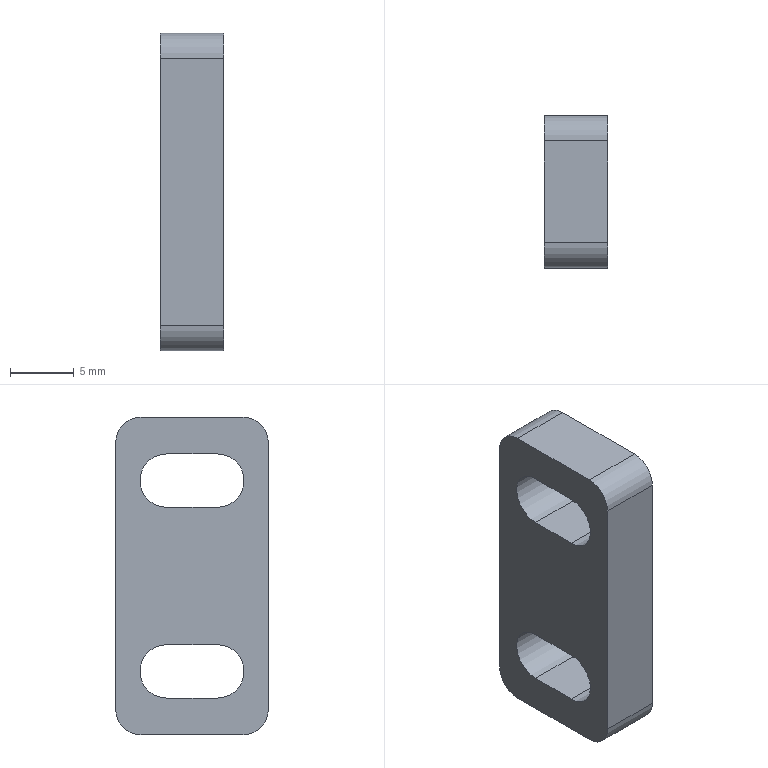Part | SolidWorks | features Fillet 4, ICE 4, Cut 1, Extrusion 1, HoleWzd 1 | 1 solid | 18 faces | box 5 x 12 x 25 mm | volume 1176 mm3 | plane 10 | cylinder 8 | commonest cylinder face diameters 4 x4 4.2 x4
STEP:
#1=CARTESIAN_POINT('',(0.,-4.,-12.5));
#2=VERTEX_POINT('',#1);
#3=CARTESIAN_POINT('',(0.,4.,-12.5));
#4=VERTEX_POINT('',#3);
#5=CARTESIAN_POINT('',(0.,6.,-12.5));
#6=DIRECTION('',(0.,1.,0.));
#7=VECTOR('',#6,1000.);
#8=LINE('',#5,#7);
#9=EDGE_CURVE('',#2,#4,#8,.T.);
#10=ORIENTED_EDGE('',*,*,#9,.T.);
#11=CARTESIAN_POINT('',(5.,4.,-12.5));
#12=VERTEX_POINT('',#11);
#13=CARTESIAN_POINT('',(5.,4.,-12.5));
#14=DIRECTION('',(1.,0.,0.));
#15=VECTOR('',#14,1000.);
#16=LINE('',#13,#15);
#17=EDGE_CURVE('',#4,#12,#16,.T.);
#18=ORIENTED_EDGE('',*,*,#17,.T.);
#19=CARTESIAN_POINT('',(5.,-4.,-12.5));
#20=VERTEX_POINT('',#19);
#21=CARTESIAN_POINT('',(5.,6.,-12.5));
#22=DIRECTION('',(0.,1.,0.));
#23=VECTOR('',#22,1000.);
#24=LINE('',#21,#23);
#25=EDGE_CURVE('',#20,#12,#24,.T.);
#26=ORIENTED_EDGE('',*,*,#25,.F.);
#27=CARTESIAN_POINT('',(5.,-4.,-12.5));
#28=DIRECTION('',(-1.,0.,0.));
#29=VECTOR('',#28,1000.);
#30=LINE('',#27,#29);
#31=EDGE_CURVE('',#20,#2,#30,.T.);
#32=ORIENTED_EDGE('',*,*,#31,.T.);
#33=EDGE_LOOP('',(#10,#18,#26,#32));
#34=FACE_OUTER_BOUND('',#33,.T.);
#35=CARTESIAN_POINT('',(5.,6.,-12.5));
#36=DIRECTION('',(0.,0.,1.));
#37=DIRECTION('',(0.,-1.,0.));
#38=AXIS2_PLACEMENT_3D('',#35,#36,#37);
#39=PLANE('',#38);
#40=ADVANCED_FACE('',(#34),#39,.F.);
#41=CARTESIAN_POINT('',(5.,4.,12.5));
#42=VERTEX_POINT('',#41);
#43=CARTESIAN_POINT('',(5.,-4.,12.5));
#44=VERTEX_POINT('',#43);
#45=CARTESIAN_POINT('',(5.,6.,12.5));
#46=DIRECTION('',(0.,-1.,0.));
#47=VECTOR('',#46,1000.);
#48=LINE('',#45,#47);
#49=EDGE_CURVE('',#42,#44,#48,.T.);
#50=ORIENTED_EDGE('',*,*,#49,.F.);
#51=CARTESIAN_POINT('',(0.,4.,12.5));
#52=VERTEX_POINT('',#51);
#53=CARTESIAN_POINT('',(5.,4.,12.5));
#54=DIRECTION('',(-1.,0.,0.));
#55=VECTOR('',#54,1000.);
#56=LINE('',#53,#55);
#57=EDGE_CURVE('',#42,#52,#56,.T.);
#58=ORIENTED_EDGE('',*,*,#57,.T.);
#59=CARTESIAN_POINT('',(0.,-4.,12.5));
#60=VERTEX_POINT('',#59);
#61=CARTESIAN_POINT('',(0.,6.,12.5));
#62=DIRECTION('',(0.,-1.,0.));
#63=VECTOR('',#62,1000.);
#64=LINE('',#61,#63);
#65=EDGE_CURVE('',#52,#60,#64,.T.);
#66=ORIENTED_EDGE('',*,*,#65,.T.);
#67=CARTESIAN_POINT('',(5.,-4.,12.5));
#68=DIRECTION('',(1.,0.,0.));
#69=VECTOR('',#68,1000.);
#70=LINE('',#67,#69);
#71=EDGE_CURVE('',#60,#44,#70,.T.);
#72=ORIENTED_EDGE('',*,*,#71,.T.);
#73=EDGE_LOOP('',(#50,#58,#66,#72));
#74=FACE_OUTER_BOUND('',#73,.T.);
#75=CARTESIAN_POINT('',(5.,6.,12.5));
#76=DIRECTION('',(0.,0.,-1.));
#77=DIRECTION('',(-1.,0.,0.));
#78=AXIS2_PLACEMENT_3D('',#75,#76,#77);
#79=PLANE('',#78);
#80=ADVANCED_FACE('',(#74),#79,.F.);
#81=CARTESIAN_POINT('',(0.,-6.,10.5));
#82=VERTEX_POINT('',#81);
#83=CARTESIAN_POINT('',(0.,-6.,-10.5));
#84=VERTEX_POINT('',#83);
#85=CARTESIAN_POINT('',(0.,-6.,12.5));
#86=DIRECTION('',(0.,0.,-1.));
#87=VECTOR('',#86,1000.);
#88=LINE('',#85,#87);
#89=EDGE_CURVE('',#82,#84,#88,.T.);
#90=ORIENTED_EDGE('',*,*,#89,.T.);
#91=CARTESIAN_POINT('',(5.,-6.,-10.5));
#92=VERTEX_POINT('',#91);
#93=CARTESIAN_POINT('',(5.,-6.,-10.5));
#94=DIRECTION('',(1.,0.,0.));
#95=VECTOR('',#94,1000.);
#96=LINE('',#93,#95);
#97=EDGE_CURVE('',#84,#92,#96,.T.);
#98=ORIENTED_EDGE('',*,*,#97,.T.);
#99=CARTESIAN_POINT('',(5.,-6.,10.5));
#100=VERTEX_POINT('',#99);
#101=CARTESIAN_POINT('',(5.,-6.,12.5));
#102=DIRECTION('',(0.,0.,-1.));
#103=VECTOR('',#102,1000.);
#104=LINE('',#101,#103);
#105=EDGE_CURVE('',#100,#92,#104,.T.);
#106=ORIENTED_EDGE('',*,*,#105,.F.);
#107=CARTESIAN_POINT('',(5.,-6.,10.5));
#108=DIRECTION('',(-1.,0.,0.));
#109=VECTOR('',#108,1000.);
#110=LINE('',#107,#109);
#111=EDGE_CURVE('',#100,#82,#110,.T.);
#112=ORIENTED_EDGE('',*,*,#111,.T.);
#113=EDGE_LOOP('',(#90,#98,#106,#112));
#114=FACE_OUTER_BOUND('',#113,.T.);
#115=CARTESIAN_POINT('',(5.,-6.,12.5));
#116=DIRECTION('',(0.,1.,0.));
#117=DIRECTION('',(0.,0.,1.));
#118=AXIS2_PLACEMENT_3D('',#115,#116,#117);
#119=PLANE('',#118);
#120=ADVANCED_FACE('',(#114),#119,.F.);
#121=CARTESIAN_POINT('',(5.,6.,10.5));
#122=VERTEX_POINT('',#121);
#123=CARTESIAN_POINT('',(5.,6.,-10.5));
#124=VERTEX_POINT('',#123);
#125=CARTESIAN_POINT('',(5.,6.,-15.392));
#126=DIRECTION('',(0.,0.,-1.));
#127=VECTOR('',#126,1000.);
#128=LINE('',#125,#127);
#129=EDGE_CURVE('',#122,#124,#128,.T.);
#130=ORIENTED_EDGE('',*,*,#129,.F.);
#131=CARTESIAN_POINT('',(5.,4.,10.5));
#132=DIRECTION('',(1.,0.,0.));
#133=DIRECTION('',(0.,0.,-1.));
#134=AXIS2_PLACEMENT_3D('',#131,#132,#133);
#135=CIRCLE('',#134,2.);
#136=EDGE_CURVE('',#122,#42,#135,.T.);
#137=ORIENTED_EDGE('',*,*,#136,.T.);
#138=ORIENTED_EDGE('',*,*,#49,.T.);
#139=CARTESIAN_POINT('',(5.,-4.,10.5));
#140=DIRECTION('',(1.,0.,0.));
#141=DIRECTION('',(0.,0.,-1.));
#142=AXIS2_PLACEMENT_3D('',#139,#140,#141);
#143=CIRCLE('',#142,2.);
#144=EDGE_CURVE('',#44,#100,#143,.T.);
#145=ORIENTED_EDGE('',*,*,#144,.T.);
#146=ORIENTED_EDGE('',*,*,#105,.T.);
#147=CARTESIAN_POINT('',(5.,-4.,-10.5));
#148=DIRECTION('',(1.,0.,0.));
#149=DIRECTION('',(0.,0.,-1.));
#150=AXIS2_PLACEMENT_3D('',#147,#148,#149);
#151=CIRCLE('',#150,2.);
#152=EDGE_CURVE('',#92,#20,#151,.T.);
#153=ORIENTED_EDGE('',*,*,#152,.T.);
#154=ORIENTED_EDGE('',*,*,#25,.T.);
#155=CARTESIAN_POINT('',(5.,4.,-10.5));
#156=DIRECTION('',(1.,0.,0.));
#157=DIRECTION('',(0.,0.,-1.));
#158=AXIS2_PLACEMENT_3D('',#155,#156,#157);
#159=CIRCLE('',#158,2.);
#160=EDGE_CURVE('',#12,#124,#159,.T.);
#161=ORIENTED_EDGE('',*,*,#160,.T.);
#162=EDGE_LOOP('',(#130,#137,#138,#145,#146,#153,#154,#161));
#163=FACE_OUTER_BOUND('',#162,.T.);
#164=CARTESIAN_POINT('',(5.,2.,5.4));
#165=VERTEX_POINT('',#164);
#166=CARTESIAN_POINT('',(5.,2.,9.6));
#167=VERTEX_POINT('',#166);
#168=CARTESIAN_POINT('',(5.,2.,7.5));
#169=DIRECTION('',(1.,0.,0.));
#170=DIRECTION('',(0.,0.,-1.));
#171=AXIS2_PLACEMENT_3D('',#168,#169,#170);
#172=CIRCLE('',#171,2.1);
#173=EDGE_CURVE('',#165,#167,#172,.T.);
#174=ORIENTED_EDGE('',*,*,#173,.F.);
#175=CARTESIAN_POINT('',(5.,-2.,5.4));
#176=VERTEX_POINT('',#175);
#177=CARTESIAN_POINT('',(5.,0.,5.4));
#178=DIRECTION('',(0.,1.,0.));
#179=VECTOR('',#178,1000.);
#180=LINE('',#177,#179);
#181=EDGE_CURVE('',#176,#165,#180,.T.);
#182=ORIENTED_EDGE('',*,*,#181,.F.);
#183=CARTESIAN_POINT('',(5.,-2.,9.6));
#184=VERTEX_POINT('',#183);
#185=CARTESIAN_POINT('',(5.,-2.,7.5));
#186=DIRECTION('',(1.,0.,0.));
#187=DIRECTION('',(0.,0.,-1.));
#188=AXIS2_PLACEMENT_3D('',#185,#186,#187);
#189=CIRCLE('',#188,2.1);
#190=EDGE_CURVE('',#184,#176,#189,.T.);
#191=ORIENTED_EDGE('',*,*,#190,.F.);
#192=CARTESIAN_POINT('',(5.,0.,9.6));
#193=DIRECTION('',(0.,-1.,0.));
#194=VECTOR('',#193,1000.);
#195=LINE('',#192,#194);
#196=EDGE_CURVE('',#167,#184,#195,.T.);
#197=ORIENTED_EDGE('',*,*,#196,.F.);
#198=EDGE_LOOP('',(#174,#182,#191,#197));
#199=FACE_BOUND('',#198,.T.);
#200=CARTESIAN_POINT('',(5.,2.,-9.6));
#201=VERTEX_POINT('',#200);
#202=CARTESIAN_POINT('',(5.,2.,-5.4));
#203=VERTEX_POINT('',#202);
#204=CARTESIAN_POINT('',(5.,2.,-7.5));
#205=DIRECTION('',(1.,0.,0.));
#206=DIRECTION('',(0.,0.,-1.));
#207=AXIS2_PLACEMENT_3D('',#204,#205,#206);
#208=CIRCLE('',#207,2.1);
#209=EDGE_CURVE('',#201,#203,#208,.T.);
#210=ORIENTED_EDGE('',*,*,#209,.F.);
#211=CARTESIAN_POINT('',(5.,-2.,-9.6));
#212=VERTEX_POINT('',#211);
#213=CARTESIAN_POINT('',(5.,0.,-9.6));
#214=DIRECTION('',(0.,1.,0.));
#215=VECTOR('',#214,1000.);
#216=LINE('',#213,#215);
#217=EDGE_CURVE('',#212,#201,#216,.T.);
#218=ORIENTED_EDGE('',*,*,#217,.F.);
#219=CARTESIAN_POINT('',(5.,-2.,-5.4));
#220=VERTEX_POINT('',#219);
#221=CARTESIAN_POINT('',(5.,-2.,-7.5));
#222=DIRECTION('',(1.,0.,0.));
#223=DIRECTION('',(0.,0.,-1.));
#224=AXIS2_PLACEMENT_3D('',#221,#222,#223);
#225=CIRCLE('',#224,2.1);
#226=EDGE_CURVE('',#220,#212,#225,.T.);
#227=ORIENTED_EDGE('',*,*,#226,.F.);
#228=CARTESIAN_POINT('',(5.,0.,-5.4));
#229=DIRECTION('',(0.,-1.,0.));
#230=VECTOR('',#229,1000.);
#231=LINE('',#228,#230);
#232=EDGE_CURVE('',#203,#220,#231,.T.);
#233=ORIENTED_EDGE('',*,*,#232,.F.);
#234=EDGE_LOOP('',(#210,#218,#227,#233));
#235=FACE_BOUND('',#234,.T.);
#236=CARTESIAN_POINT('',(5.,0.,0.));
#237=DIRECTION('',(1.,0.,0.));
#238=DIRECTION('',(0.,0.,-1.));
#239=AXIS2_PLACEMENT_3D('',#236,#237,#238);
#240=PLANE('',#239);
#241=ADVANCED_FACE('',(#163,#199,#235),#240,.T.);
#242=CARTESIAN_POINT('',(0.,2.,5.4));
#243=VERTEX_POINT('',#242);
#244=CARTESIAN_POINT('',(0.,-2.,5.4));
#245=VERTEX_POINT('',#244);
#246=CARTESIAN_POINT('',(0.,2.,5.4));
#247=DIRECTION('',(0.,-1.,0.));
#248=VECTOR('',#247,1000.);
#249=LINE('',#246,#248);
#250=EDGE_CURVE('',#243,#245,#249,.T.);
#251=ORIENTED_EDGE('',*,*,#250,.F.);
#252=CARTESIAN_POINT('',(0.,2.,9.6));
#253=VERTEX_POINT('',#252);
#254=CARTESIAN_POINT('',(0.,2.,7.5));
#255=DIRECTION('',(-1.,0.,0.));
#256=DIRECTION('',(0.,0.,-1.));
#257=AXIS2_PLACEMENT_3D('',#254,#255,#256);
#258=CIRCLE('',#257,2.1);
#259=EDGE_CURVE('',#253,#243,#258,.T.);
#260=ORIENTED_EDGE('',*,*,#259,.F.);
#261=CARTESIAN_POINT('',(0.,-2.,9.6));
#262=VERTEX_POINT('',#261);
#263=CARTESIAN_POINT('',(0.,2.,9.6));
#264=DIRECTION('',(0.,1.,0.));
#265=VECTOR('',#264,1000.);
#266=LINE('',#263,#265);
#267=EDGE_CURVE('',#262,#253,#266,.T.);
#268=ORIENTED_EDGE('',*,*,#267,.F.);
#269=CARTESIAN_POINT('',(0.,-2.,7.5));
#270=DIRECTION('',(-1.,0.,0.));
#271=DIRECTION('',(0.,0.,-1.));
#272=AXIS2_PLACEMENT_3D('',#269,#270,#271);
#273=CIRCLE('',#272,2.1);
#274=EDGE_CURVE('',#245,#262,#273,.T.);
#275=ORIENTED_EDGE('',*,*,#274,.F.);
#276=EDGE_LOOP('',(#251,#260,#268,#275));
#277=FACE_BOUND('',#276,.T.);
#278=CARTESIAN_POINT('',(0.,2.,-9.6));
#279=VERTEX_POINT('',#278);
#280=CARTESIAN_POINT('',(0.,-2.,-9.6));
#281=VERTEX_POINT('',#280);
#282=CARTESIAN_POINT('',(0.,2.,-9.6));
#283=DIRECTION('',(0.,-1.,0.));
#284=VECTOR('',#283,1000.);
#285=LINE('',#282,#284);
#286=EDGE_CURVE('',#279,#281,#285,.T.);
#287=ORIENTED_EDGE('',*,*,#286,.F.);
#288=CARTESIAN_POINT('',(0.,2.,-5.4));
#289=VERTEX_POINT('',#288);
#290=CARTESIAN_POINT('',(0.,2.,-7.5));
#291=DIRECTION('',(-1.,0.,0.));
#292=DIRECTION('',(0.,0.,1.));
#293=AXIS2_PLACEMENT_3D('',#290,#291,#292);
#294=CIRCLE('',#293,2.1);
#295=EDGE_CURVE('',#289,#279,#294,.T.);
#296=ORIENTED_EDGE('',*,*,#295,.F.);
#297=CARTESIAN_POINT('',(0.,-2.,-5.4));
#298=VERTEX_POINT('',#297);
#299=CARTESIAN_POINT('',(0.,2.,-5.4));
#300=DIRECTION('',(0.,1.,0.));
#301=VECTOR('',#300,1000.);
#302=LINE('',#299,#301);
#303=EDGE_CURVE('',#298,#289,#302,.T.);
#304=ORIENTED_EDGE('',*,*,#303,.F.);
#305=CARTESIAN_POINT('',(0.,-2.,-7.5));
#306=DIRECTION('',(-1.,0.,0.));
#307=DIRECTION('',(0.,0.,1.));
#308=AXIS2_PLACEMENT_3D('',#305,#306,#307);
#309=CIRCLE('',#308,2.1);
#310=EDGE_CURVE('',#281,#298,#309,.T.);
#311=ORIENTED_EDGE('',*,*,#310,.F.);
#312=EDGE_LOOP('',(#287,#296,#304,#311));
#313=FACE_BOUND('',#312,.T.);
#314=ORIENTED_EDGE('',*,*,#65,.F.);
#315=CARTESIAN_POINT('',(0.,6.,10.5));
#316=VERTEX_POINT('',#315);
#317=CARTESIAN_POINT('',(0.,4.,10.5));
#318=DIRECTION('',(-1.,0.,0.));
#319=DIRECTION('',(0.,0.,-1.));
#320=AXIS2_PLACEMENT_3D('',#317,#318,#319);
#321=CIRCLE('',#320,2.);
#322=EDGE_CURVE('',#52,#316,#321,.T.);
#323=ORIENTED_EDGE('',*,*,#322,.T.);
#324=CARTESIAN_POINT('',(0.,6.,-10.5));
#325=VERTEX_POINT('',#324);
#326=CARTESIAN_POINT('',(0.,6.,0.));
#327=DIRECTION('',(0.,0.,-1.));
#328=VECTOR('',#327,1000.);
#329=LINE('',#326,#328);
#330=EDGE_CURVE('',#316,#325,#329,.T.);
#331=ORIENTED_EDGE('',*,*,#330,.T.);
#332=CARTESIAN_POINT('',(0.,4.,-10.5));
#333=DIRECTION('',(-1.,0.,0.));
#334=DIRECTION('',(0.,0.,-1.));
#335=AXIS2_PLACEMENT_3D('',#332,#333,#334);
#336=CIRCLE('',#335,2.);
#337=EDGE_CURVE('',#325,#4,#336,.T.);
#338=ORIENTED_EDGE('',*,*,#337,.T.);
#339=ORIENTED_EDGE('',*,*,#9,.F.);
#340=CARTESIAN_POINT('',(0.,-4.,-10.5));
#341=DIRECTION('',(-1.,0.,0.));
#342=DIRECTION('',(0.,0.,-1.));
#343=AXIS2_PLACEMENT_3D('',#340,#341,#342);
#344=CIRCLE('',#343,2.);
#345=EDGE_CURVE('',#2,#84,#344,.T.);
#346=ORIENTED_EDGE('',*,*,#345,.T.);
#347=ORIENTED_EDGE('',*,*,#89,.F.);
#348=CARTESIAN_POINT('',(0.,-4.,10.5));
#349=DIRECTION('',(-1.,0.,0.));
#350=DIRECTION('',(0.,0.,-1.));
#351=AXIS2_PLACEMENT_3D('',#348,#349,#350);
#352=CIRCLE('',#351,2.);
#353=EDGE_CURVE('',#82,#60,#352,.T.);
#354=ORIENTED_EDGE('',*,*,#353,.T.);
#355=EDGE_LOOP('',(#314,#323,#331,#338,#339,#346,#347,#354));
#356=FACE_OUTER_BOUND('',#355,.T.);
#357=CARTESIAN_POINT('',(0.,0.,0.));
#358=DIRECTION('',(1.,0.,0.));
#359=DIRECTION('',(0.,0.,-1.));
#360=AXIS2_PLACEMENT_3D('',#357,#358,#359);
#361=PLANE('',#360);
#362=ADVANCED_FACE('',(#277,#313,#356),#361,.F.);
#363=ORIENTED_EDGE('',*,*,#209,.T.);
#364=CARTESIAN_POINT('',(13.,2.,-5.4));
#365=DIRECTION('',(-1.,0.,0.));
#366=VECTOR('',#365,1000.);
#367=LINE('',#364,#366);
#368=EDGE_CURVE('',#203,#289,#367,.T.);
#369=ORIENTED_EDGE('',*,*,#368,.T.);
#370=ORIENTED_EDGE('',*,*,#295,.T.);
#371=CARTESIAN_POINT('',(13.,2.,-9.6));
#372=DIRECTION('',(-1.,0.,0.));
#373=VECTOR('',#372,1000.);
#374=LINE('',#371,#373);
#375=EDGE_CURVE('',#201,#279,#374,.T.);
#376=ORIENTED_EDGE('',*,*,#375,.F.);
#377=EDGE_LOOP('',(#363,#369,#370,#376));
#378=FACE_OUTER_BOUND('',#377,.T.);
#379=CARTESIAN_POINT('',(13.,2.,-7.5));
#380=DIRECTION('',(-1.,0.,0.));
#381=DIRECTION('',(0.,0.,1.));
#382=AXIS2_PLACEMENT_3D('',#379,#380,#381);
#383=CYLINDRICAL_SURFACE('',#382,2.1);
#384=ADVANCED_FACE('',(#378),#383,.F.);
#385=ORIENTED_EDGE('',*,*,#232,.T.);
#386=CARTESIAN_POINT('',(13.,-2.,-5.4));
#387=DIRECTION('',(-1.,0.,0.));
#388=VECTOR('',#387,1000.);
#389=LINE('',#386,#388);
#390=EDGE_CURVE('',#220,#298,#389,.T.);
#391=ORIENTED_EDGE('',*,*,#390,.T.);
#392=ORIENTED_EDGE('',*,*,#303,.T.);
#393=ORIENTED_EDGE('',*,*,#368,.F.);
#394=EDGE_LOOP('',(#385,#391,#392,#393));
#395=FACE_OUTER_BOUND('',#394,.T.);
#396=CARTESIAN_POINT('',(13.,2.,-5.4));
#397=DIRECTION('',(0.,0.,1.));
#398=DIRECTION('',(1.,0.,0.));
#399=AXIS2_PLACEMENT_3D('',#396,#397,#398);
#400=PLANE('',#399);
#401=ADVANCED_FACE('',(#395),#400,.F.);
#402=ORIENTED_EDGE('',*,*,#226,.T.);
#403=CARTESIAN_POINT('',(13.,-2.,-9.6));
#404=DIRECTION('',(-1.,0.,0.));
#405=VECTOR('',#404,1000.);
#406=LINE('',#403,#405);
#407=EDGE_CURVE('',#212,#281,#406,.T.);
#408=ORIENTED_EDGE('',*,*,#407,.T.);
#409=ORIENTED_EDGE('',*,*,#310,.T.);
#410=ORIENTED_EDGE('',*,*,#390,.F.);
#411=EDGE_LOOP('',(#402,#408,#409,#410));
#412=FACE_OUTER_BOUND('',#411,.T.);
#413=CARTESIAN_POINT('',(13.,-2.,-7.5));
#414=DIRECTION('',(-1.,0.,0.));
#415=DIRECTION('',(0.,0.,1.));
#416=AXIS2_PLACEMENT_3D('',#413,#414,#415);
#417=CYLINDRICAL_SURFACE('',#416,2.1);
#418=ADVANCED_FACE('',(#412),#417,.F.);
#419=ORIENTED_EDGE('',*,*,#217,.T.);
#420=ORIENTED_EDGE('',*,*,#375,.T.);
#421=ORIENTED_EDGE('',*,*,#286,.T.);
#422=ORIENTED_EDGE('',*,*,#407,.F.);
#423=EDGE_LOOP('',(#419,#420,#421,#422));
#424=FACE_OUTER_BOUND('',#423,.T.);
#425=CARTESIAN_POINT('',(13.,2.,-9.6));
#426=DIRECTION('',(0.,0.,-1.));
#427=DIRECTION('',(-1.,0.,0.));
#428=AXIS2_PLACEMENT_3D('',#425,#426,#427);
#429=PLANE('',#428);
#430=ADVANCED_FACE('',(#424),#429,.F.);
#431=ORIENTED_EDGE('',*,*,#173,.T.);
#432=CARTESIAN_POINT('',(13.,2.,9.6));
#433=DIRECTION('',(-1.,0.,0.));
#434=VECTOR('',#433,1000.);
#435=LINE('',#432,#434);
#436=EDGE_CURVE('',#167,#253,#435,.T.);
#437=ORIENTED_EDGE('',*,*,#436,.T.);
#438=ORIENTED_EDGE('',*,*,#259,.T.);
#439=CARTESIAN_POINT('',(13.,2.,5.4));
#440=DIRECTION('',(-1.,0.,0.));
#441=VECTOR('',#440,1000.);
#442=LINE('',#439,#441);
#443=EDGE_CURVE('',#165,#243,#442,.T.);
#444=ORIENTED_EDGE('',*,*,#443,.F.);
#445=EDGE_LOOP('',(#431,#437,#438,#444));
#446=FACE_OUTER_BOUND('',#445,.T.);
#447=CARTESIAN_POINT('',(13.,2.,7.5));
#448=DIRECTION('',(-1.,0.,0.));
#449=DIRECTION('',(0.,0.,1.));
#450=AXIS2_PLACEMENT_3D('',#447,#448,#449);
#451=CYLINDRICAL_SURFACE('',#450,2.1);
#452=ADVANCED_FACE('',(#446),#451,.F.);
#453=ORIENTED_EDGE('',*,*,#196,.T.);
#454=CARTESIAN_POINT('',(13.,-2.,9.6));
#455=DIRECTION('',(-1.,0.,0.));
#456=VECTOR('',#455,1000.);
#457=LINE('',#454,#456);
#458=EDGE_CURVE('',#184,#262,#457,.T.);
#459=ORIENTED_EDGE('',*,*,#458,.T.);
#460=ORIENTED_EDGE('',*,*,#267,.T.);
#461=ORIENTED_EDGE('',*,*,#436,.F.);
#462=EDGE_LOOP('',(#453,#459,#460,#461));
#463=FACE_OUTER_BOUND('',#462,.T.);
#464=CARTESIAN_POINT('',(13.,2.,9.6));
#465=DIRECTION('',(0.,0.,1.));
#466=DIRECTION('',(1.,0.,0.));
#467=AXIS2_PLACEMENT_3D('',#464,#465,#466);
#468=PLANE('',#467);
#469=ADVANCED_FACE('',(#463),#468,.F.);
#470=ORIENTED_EDGE('',*,*,#190,.T.);
#471=CARTESIAN_POINT('',(13.,-2.,5.4));
#472=DIRECTION('',(-1.,0.,0.));
#473=VECTOR('',#472,1000.);
#474=LINE('',#471,#473);
#475=EDGE_CURVE('',#176,#245,#474,.T.);
#476=ORIENTED_EDGE('',*,*,#475,.T.);
#477=ORIENTED_EDGE('',*,*,#274,.T.);
#478=ORIENTED_EDGE('',*,*,#458,.F.);
#479=EDGE_LOOP('',(#470,#476,#477,#478));
#480=FACE_OUTER_BOUND('',#479,.T.);
#481=CARTESIAN_POINT('',(13.,-2.,7.5));
#482=DIRECTION('',(-1.,0.,0.));
#483=DIRECTION('',(0.,0.,1.));
#484=AXIS2_PLACEMENT_3D('',#481,#482,#483);
#485=CYLINDRICAL_SURFACE('',#484,2.1);
#486=ADVANCED_FACE('',(#480),#485,.F.);
#487=ORIENTED_EDGE('',*,*,#181,.T.);
#488=ORIENTED_EDGE('',*,*,#443,.T.);
#489=ORIENTED_EDGE('',*,*,#250,.T.);
#490=ORIENTED_EDGE('',*,*,#475,.F.);
#491=EDGE_LOOP('',(#487,#488,#489,#490));
#492=FACE_OUTER_BOUND('',#491,.T.);
#493=CARTESIAN_POINT('',(13.,2.,5.4));
#494=DIRECTION('',(0.,0.,-1.));
#495=DIRECTION('',(-1.,0.,0.));
#496=AXIS2_PLACEMENT_3D('',#493,#494,#495);
#497=PLANE('',#496);
#498=ADVANCED_FACE('',(#492),#497,.F.);
#499=ORIENTED_EDGE('',*,*,#152,.F.);
#500=ORIENTED_EDGE('',*,*,#97,.F.);
#501=ORIENTED_EDGE('',*,*,#345,.F.);
#502=ORIENTED_EDGE('',*,*,#31,.F.);
#503=EDGE_LOOP('',(#499,#500,#501,#502));
#504=FACE_OUTER_BOUND('',#503,.T.);
#505=CARTESIAN_POINT('',(5.,-4.,-10.5));
#506=DIRECTION('',(-1.,0.,0.));
#507=DIRECTION('',(0.,0.,1.));
#508=AXIS2_PLACEMENT_3D('',#505,#506,#507);
#509=CYLINDRICAL_SURFACE('',#508,2.);
#510=ADVANCED_FACE('',(#504),#509,.T.);
#511=ORIENTED_EDGE('',*,*,#144,.F.);
#512=ORIENTED_EDGE('',*,*,#71,.F.);
#513=ORIENTED_EDGE('',*,*,#353,.F.);
#514=ORIENTED_EDGE('',*,*,#111,.F.);
#515=EDGE_LOOP('',(#511,#512,#513,#514));
#516=FACE_OUTER_BOUND('',#515,.T.);
#517=CARTESIAN_POINT('',(5.,-4.,10.5));
#518=DIRECTION('',(-1.,0.,0.));
#519=DIRECTION('',(0.,0.,1.));
#520=AXIS2_PLACEMENT_3D('',#517,#518,#519);
#521=CYLINDRICAL_SURFACE('',#520,2.);
#522=ADVANCED_FACE('',(#516),#521,.T.);
#523=ORIENTED_EDGE('',*,*,#330,.F.);
#524=CARTESIAN_POINT('',(-16.,6.,10.5));
#525=DIRECTION('',(1.,0.,0.));
#526=VECTOR('',#525,1000.);
#527=LINE('',#524,#526);
#528=EDGE_CURVE('',#316,#122,#527,.T.);
#529=ORIENTED_EDGE('',*,*,#528,.T.);
#530=ORIENTED_EDGE('',*,*,#129,.T.);
#531=CARTESIAN_POINT('',(-16.,6.,-10.5));
#532=DIRECTION('',(-1.,0.,0.));
#533=VECTOR('',#532,1000.);
#534=LINE('',#531,#533);
#535=EDGE_CURVE('',#124,#325,#534,.T.);
#536=ORIENTED_EDGE('',*,*,#535,.T.);
#537=EDGE_LOOP('',(#523,#529,#530,#536));
#538=FACE_OUTER_BOUND('',#537,.T.);
#539=CARTESIAN_POINT('',(-16.,6.,-15.392));
#540=DIRECTION('',(0.,-1.,0.));
#541=DIRECTION('',(0.,0.,-1.));
#542=AXIS2_PLACEMENT_3D('',#539,#540,#541);
#543=PLANE('',#542);
#544=ADVANCED_FACE('',(#538),#543,.F.);
#545=ORIENTED_EDGE('',*,*,#136,.F.);
#546=ORIENTED_EDGE('',*,*,#528,.F.);
#547=ORIENTED_EDGE('',*,*,#322,.F.);
#548=ORIENTED_EDGE('',*,*,#57,.F.);
#549=EDGE_LOOP('',(#545,#546,#547,#548));
#550=FACE_OUTER_BOUND('',#549,.T.);
#551=CARTESIAN_POINT('',(5.,4.,10.5));
#552=DIRECTION('',(-1.,0.,0.));
#553=DIRECTION('',(0.,0.,1.));
#554=AXIS2_PLACEMENT_3D('',#551,#552,#553);
#555=CYLINDRICAL_SURFACE('',#554,2.);
#556=ADVANCED_FACE('',(#550),#555,.T.);
#557=ORIENTED_EDGE('',*,*,#160,.F.);
#558=ORIENTED_EDGE('',*,*,#17,.F.);
#559=ORIENTED_EDGE('',*,*,#337,.F.);
#560=ORIENTED_EDGE('',*,*,#535,.F.);
#561=EDGE_LOOP('',(#557,#558,#559,#560));
#562=FACE_OUTER_BOUND('',#561,.T.);
#563=CARTESIAN_POINT('',(-16.,4.,-10.5));
#564=DIRECTION('',(-1.,0.,0.));
#565=DIRECTION('',(0.,0.,1.));
#566=AXIS2_PLACEMENT_3D('',#563,#564,#565);
#567=CYLINDRICAL_SURFACE('',#566,2.);
#568=ADVANCED_FACE('',(#562),#567,.T.);
#569=CLOSED_SHELL('',(#40,#80,#120,#241,#362,#384,#401,#418,#430,#452,#469,#486,#498,#510,#522,#544,#556,#568));
#570=MANIFOLD_SOLID_BREP('',#569);
#571=CARTESIAN_POINT('',(0.,0.,0.));
#572=DIRECTION('',(0.,0.,1.));
#573=DIRECTION('',(1.,0.,0.));
#574=AXIS2_PLACEMENT_3D('',#571,#572,#573);
#575=(LENGTH_UNIT()NAMED_UNIT(*)SI_UNIT(.MILLI.,.METRE.));
#576=UNCERTAINTY_MEASURE_WITH_UNIT(LENGTH_MEASURE(0.00001),#575,'','');
#577=(NAMED_UNIT(*)PLANE_ANGLE_UNIT()SI_UNIT($,.RADIAN.));
#578=(NAMED_UNIT(*)SI_UNIT($,.STERADIAN.)SOLID_ANGLE_UNIT());
#579=(GEOMETRIC_REPRESENTATION_CONTEXT(3)GLOBAL_UNCERTAINTY_ASSIGNED_CONTEXT((#576))GLOBAL_UNIT_ASSIGNED_CONTEXT((#575,#577,#578))REPRESENTATION_CONTEXT('',''));
#580=ADVANCED_BREP_SHAPE_REPRESENTATION('',(#570,#574),#579);